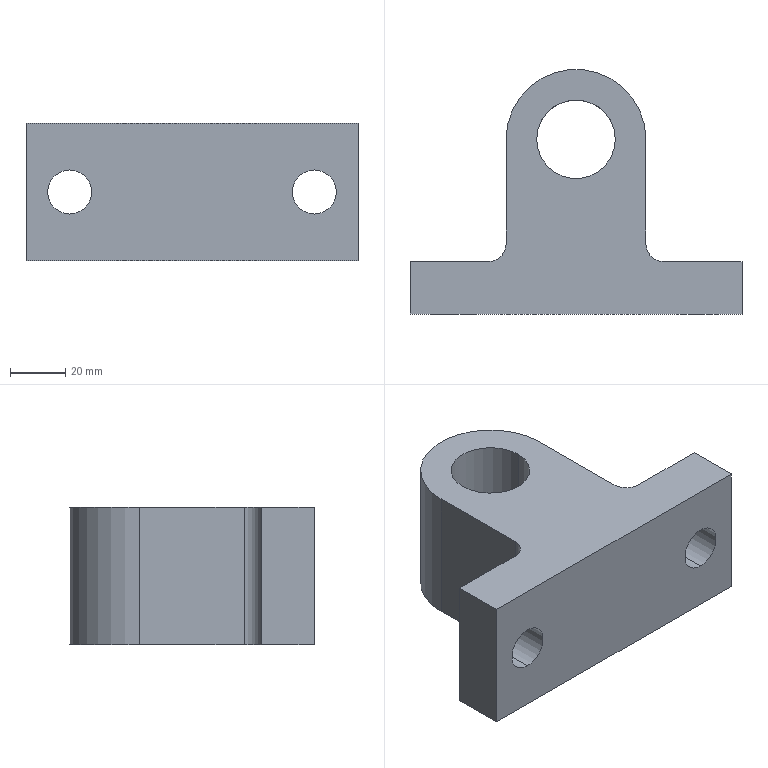Part | SolidWorks | features Cut 1, Extrusion 1, Fillet 1 | 1 solid | 18 faces | box 120.65 x 88.9 x 50 mm | volume 239631 mm3 | cylinder 9 | plane 9 | commonest cylinder face diameters 16.002 x4 12.7 x2 28.575 x2 50.8 x1
STEP:
#1=CARTESIAN_POINT('',(-44.45,-63.5,-8.001));
#2=VERTEX_POINT('',#1);
#3=CARTESIAN_POINT('',(-44.45,-63.5,8.001));
#4=VERTEX_POINT('',#3);
#5=CARTESIAN_POINT('',(-44.45,-63.5,0.));
#6=DIRECTION('',(0.,1.,0.));
#7=DIRECTION('',(0.,0.,-1.));
#8=AXIS2_PLACEMENT_3D('',#5,#6,#7);
#9=CIRCLE('',#8,8.001);
#10=EDGE_CURVE('',#2,#4,#9,.T.);
#11=ORIENTED_EDGE('',*,*,#10,.F.);
#12=CARTESIAN_POINT('',(-44.45,-44.45,-8.001));
#13=VERTEX_POINT('',#12);
#14=CARTESIAN_POINT('',(-44.45,-63.5,-8.001));
#15=DIRECTION('',(0.,1.,0.));
#16=VECTOR('',#15,1000.);
#17=LINE('',#14,#16);
#18=EDGE_CURVE('',#2,#13,#17,.T.);
#19=ORIENTED_EDGE('',*,*,#18,.T.);
#20=CARTESIAN_POINT('',(-44.45,-44.45,8.001));
#21=VERTEX_POINT('',#20);
#22=CARTESIAN_POINT('',(-44.45,-44.45,0.));
#23=DIRECTION('',(0.,-1.,0.));
#24=DIRECTION('',(0.,0.,-1.));
#25=AXIS2_PLACEMENT_3D('',#22,#23,#24);
#26=CIRCLE('',#25,8.001);
#27=EDGE_CURVE('',#21,#13,#26,.T.);
#28=ORIENTED_EDGE('',*,*,#27,.F.);
#29=CARTESIAN_POINT('',(-44.45,-63.5,8.001));
#30=DIRECTION('',(0.,1.,0.));
#31=VECTOR('',#30,1000.);
#32=LINE('',#29,#31);
#33=EDGE_CURVE('',#4,#21,#32,.T.);
#34=ORIENTED_EDGE('',*,*,#33,.F.);
#35=EDGE_LOOP('',(#11,#19,#28,#34));
#36=FACE_OUTER_BOUND('',#35,.T.);
#37=CARTESIAN_POINT('',(-44.45,-63.5,0.));
#38=DIRECTION('',(0.,1.,0.));
#39=DIRECTION('',(0.,0.,1.));
#40=AXIS2_PLACEMENT_3D('',#37,#38,#39);
#41=CYLINDRICAL_SURFACE('',#40,8.001);
#42=ADVANCED_FACE('',(#36),#41,.F.);
#43=CARTESIAN_POINT('',(44.45,-63.5,-8.001));
#44=VERTEX_POINT('',#43);
#45=CARTESIAN_POINT('',(44.45,-63.5,8.001));
#46=VERTEX_POINT('',#45);
#47=CARTESIAN_POINT('',(44.45,-63.5,0.));
#48=DIRECTION('',(0.,1.,0.));
#49=DIRECTION('',(0.,0.,1.));
#50=AXIS2_PLACEMENT_3D('',#47,#48,#49);
#51=CIRCLE('',#50,8.001);
#52=EDGE_CURVE('',#44,#46,#51,.T.);
#53=ORIENTED_EDGE('',*,*,#52,.F.);
#54=CARTESIAN_POINT('',(44.45,-44.45,-8.001));
#55=VERTEX_POINT('',#54);
#56=CARTESIAN_POINT('',(44.45,-63.5,-8.001));
#57=DIRECTION('',(0.,1.,0.));
#58=VECTOR('',#57,1000.);
#59=LINE('',#56,#58);
#60=EDGE_CURVE('',#44,#55,#59,.T.);
#61=ORIENTED_EDGE('',*,*,#60,.T.);
#62=CARTESIAN_POINT('',(44.45,-44.45,8.001));
#63=VERTEX_POINT('',#62);
#64=CARTESIAN_POINT('',(44.45,-44.45,0.));
#65=DIRECTION('',(0.,-1.,0.));
#66=DIRECTION('',(1.,0.,0.));
#67=AXIS2_PLACEMENT_3D('',#64,#65,#66);
#68=CIRCLE('',#67,8.001);
#69=EDGE_CURVE('',#63,#55,#68,.T.);
#70=ORIENTED_EDGE('',*,*,#69,.F.);
#71=CARTESIAN_POINT('',(44.45,-63.5,8.001));
#72=DIRECTION('',(0.,1.,0.));
#73=VECTOR('',#72,1000.);
#74=LINE('',#71,#73);
#75=EDGE_CURVE('',#46,#63,#74,.T.);
#76=ORIENTED_EDGE('',*,*,#75,.F.);
#77=EDGE_LOOP('',(#53,#61,#70,#76));
#78=FACE_OUTER_BOUND('',#77,.T.);
#79=CARTESIAN_POINT('',(44.45,-63.5,0.));
#80=DIRECTION('',(0.,1.,0.));
#81=DIRECTION('',(0.,0.,1.));
#82=AXIS2_PLACEMENT_3D('',#79,#80,#81);
#83=CYLINDRICAL_SURFACE('',#82,8.001);
#84=ADVANCED_FACE('',(#78),#83,.F.);
#85=CARTESIAN_POINT('',(-14.288,0.,25.));
#86=VERTEX_POINT('',#85);
#87=CARTESIAN_POINT('',(14.288,0.,25.));
#88=VERTEX_POINT('',#87);
#89=CARTESIAN_POINT('',(0.,0.,25.));
#90=DIRECTION('',(0.,0.,1.));
#91=DIRECTION('',(1.,0.,0.));
#92=AXIS2_PLACEMENT_3D('',#89,#90,#91);
#93=CIRCLE('',#92,14.288);
#94=EDGE_CURVE('',#86,#88,#93,.T.);
#95=ORIENTED_EDGE('',*,*,#94,.T.);
#96=CARTESIAN_POINT('',(14.288,0.,-25.));
#97=VERTEX_POINT('',#96);
#98=CARTESIAN_POINT('',(14.288,0.,25.));
#99=DIRECTION('',(0.,0.,-1.));
#100=VECTOR('',#99,1000.);
#101=LINE('',#98,#100);
#102=EDGE_CURVE('',#88,#97,#101,.T.);
#103=ORIENTED_EDGE('',*,*,#102,.T.);
#104=CARTESIAN_POINT('',(-14.288,0.,-25.));
#105=VERTEX_POINT('',#104);
#106=CARTESIAN_POINT('',(0.,0.,-25.));
#107=DIRECTION('',(0.,0.,1.));
#108=DIRECTION('',(1.,0.,0.));
#109=AXIS2_PLACEMENT_3D('',#106,#107,#108);
#110=CIRCLE('',#109,14.288);
#111=EDGE_CURVE('',#105,#97,#110,.T.);
#112=ORIENTED_EDGE('',*,*,#111,.F.);
#113=CARTESIAN_POINT('',(-14.288,0.,25.));
#114=DIRECTION('',(0.,0.,-1.));
#115=VECTOR('',#114,1000.);
#116=LINE('',#113,#115);
#117=EDGE_CURVE('',#86,#105,#116,.T.);
#118=ORIENTED_EDGE('',*,*,#117,.F.);
#119=EDGE_LOOP('',(#95,#103,#112,#118));
#120=FACE_OUTER_BOUND('',#119,.T.);
#121=CARTESIAN_POINT('',(0.,0.,25.));
#122=DIRECTION('',(0.,0.,-1.));
#123=DIRECTION('',(-1.,0.,0.));
#124=AXIS2_PLACEMENT_3D('',#121,#122,#123);
#125=CYLINDRICAL_SURFACE('',#124,14.288);
#126=ADVANCED_FACE('',(#120),#125,.F.);
#127=CARTESIAN_POINT('',(25.4,0.,25.));
#128=VERTEX_POINT('',#127);
#129=CARTESIAN_POINT('',(-25.4,0.,25.));
#130=VERTEX_POINT('',#129);
#131=CARTESIAN_POINT('',(0.,0.,25.));
#132=DIRECTION('',(0.,0.,1.));
#133=DIRECTION('',(1.,0.,0.));
#134=AXIS2_PLACEMENT_3D('',#131,#132,#133);
#135=CIRCLE('',#134,25.4);
#136=EDGE_CURVE('',#128,#130,#135,.T.);
#137=ORIENTED_EDGE('',*,*,#136,.T.);
#138=CARTESIAN_POINT('',(-25.4,-38.1,25.));
#139=VERTEX_POINT('',#138);
#140=CARTESIAN_POINT('',(-25.4,0.,25.));
#141=DIRECTION('',(0.,-1.,0.));
#142=VECTOR('',#141,1000.);
#143=LINE('',#140,#142);
#144=EDGE_CURVE('',#130,#139,#143,.T.);
#145=ORIENTED_EDGE('',*,*,#144,.T.);
#146=CARTESIAN_POINT('',(-31.75,-44.45,25.));
#147=VERTEX_POINT('',#146);
#148=CARTESIAN_POINT('',(-31.75,-38.1,25.));
#149=DIRECTION('',(0.,0.,-1.));
#150=DIRECTION('',(1.,0.,0.));
#151=AXIS2_PLACEMENT_3D('',#148,#149,#150);
#152=CIRCLE('',#151,6.35);
#153=EDGE_CURVE('',#139,#147,#152,.T.);
#154=ORIENTED_EDGE('',*,*,#153,.T.);
#155=CARTESIAN_POINT('',(-60.325,-44.45,25.));
#156=VERTEX_POINT('',#155);
#157=CARTESIAN_POINT('',(-25.4,-44.45,25.));
#158=DIRECTION('',(-1.,0.,0.));
#159=VECTOR('',#158,1000.);
#160=LINE('',#157,#159);
#161=EDGE_CURVE('',#147,#156,#160,.T.);
#162=ORIENTED_EDGE('',*,*,#161,.T.);
#163=CARTESIAN_POINT('',(-60.325,-63.5,25.));
#164=VERTEX_POINT('',#163);
#165=CARTESIAN_POINT('',(-60.325,-44.45,25.));
#166=DIRECTION('',(0.,-1.,0.));
#167=VECTOR('',#166,1000.);
#168=LINE('',#165,#167);
#169=EDGE_CURVE('',#156,#164,#168,.T.);
#170=ORIENTED_EDGE('',*,*,#169,.T.);
#171=CARTESIAN_POINT('',(60.325,-63.5,25.));
#172=VERTEX_POINT('',#171);
#173=CARTESIAN_POINT('',(-60.325,-63.5,25.));
#174=DIRECTION('',(1.,0.,0.));
#175=VECTOR('',#174,1000.);
#176=LINE('',#173,#175);
#177=EDGE_CURVE('',#164,#172,#176,.T.);
#178=ORIENTED_EDGE('',*,*,#177,.T.);
#179=CARTESIAN_POINT('',(60.325,-44.45,25.));
#180=VERTEX_POINT('',#179);
#181=CARTESIAN_POINT('',(60.325,-44.45,25.));
#182=DIRECTION('',(0.,1.,0.));
#183=VECTOR('',#182,1000.);
#184=LINE('',#181,#183);
#185=EDGE_CURVE('',#172,#180,#184,.T.);
#186=ORIENTED_EDGE('',*,*,#185,.T.);
#187=CARTESIAN_POINT('',(31.75,-44.45,25.));
#188=VERTEX_POINT('',#187);
#189=CARTESIAN_POINT('',(25.4,-44.45,25.));
#190=DIRECTION('',(-1.,0.,0.));
#191=VECTOR('',#190,1000.);
#192=LINE('',#189,#191);
#193=EDGE_CURVE('',#180,#188,#192,.T.);
#194=ORIENTED_EDGE('',*,*,#193,.T.);
#195=CARTESIAN_POINT('',(25.4,-38.1,25.));
#196=VERTEX_POINT('',#195);
#197=CARTESIAN_POINT('',(31.75,-38.1,25.));
#198=DIRECTION('',(0.,0.,-1.));
#199=DIRECTION('',(1.,0.,0.));
#200=AXIS2_PLACEMENT_3D('',#197,#198,#199);
#201=CIRCLE('',#200,6.35);
#202=EDGE_CURVE('',#188,#196,#201,.T.);
#203=ORIENTED_EDGE('',*,*,#202,.T.);
#204=CARTESIAN_POINT('',(25.4,0.,25.));
#205=DIRECTION('',(0.,1.,0.));
#206=VECTOR('',#205,1000.);
#207=LINE('',#204,#206);
#208=EDGE_CURVE('',#196,#128,#207,.T.);
#209=ORIENTED_EDGE('',*,*,#208,.T.);
#210=EDGE_LOOP('',(#137,#145,#154,#162,#170,#178,#186,#194,#203,#209));
#211=FACE_OUTER_BOUND('',#210,.T.);
#212=ORIENTED_EDGE('',*,*,#94,.F.);
#213=CARTESIAN_POINT('',(0.,0.,25.));
#214=DIRECTION('',(0.,0.,1.));
#215=DIRECTION('',(1.,0.,0.));
#216=AXIS2_PLACEMENT_3D('',#213,#214,#215);
#217=CIRCLE('',#216,14.288);
#218=EDGE_CURVE('',#88,#86,#217,.T.);
#219=ORIENTED_EDGE('',*,*,#218,.F.);
#220=EDGE_LOOP('',(#212,#219));
#221=FACE_BOUND('',#220,.T.);
#222=CARTESIAN_POINT('',(0.,0.,25.));
#223=DIRECTION('',(0.,0.,1.));
#224=DIRECTION('',(1.,0.,0.));
#225=AXIS2_PLACEMENT_3D('',#222,#223,#224);
#226=PLANE('',#225);
#227=ADVANCED_FACE('',(#211,#221),#226,.T.);
#228=CARTESIAN_POINT('',(25.4,0.,-25.));
#229=VERTEX_POINT('',#228);
#230=CARTESIAN_POINT('',(-25.4,0.,-25.));
#231=VERTEX_POINT('',#230);
#232=CARTESIAN_POINT('',(0.,0.,-25.));
#233=DIRECTION('',(0.,0.,1.));
#234=DIRECTION('',(1.,0.,0.));
#235=AXIS2_PLACEMENT_3D('',#232,#233,#234);
#236=CIRCLE('',#235,25.4);
#237=EDGE_CURVE('',#229,#231,#236,.T.);
#238=ORIENTED_EDGE('',*,*,#237,.F.);
#239=CARTESIAN_POINT('',(25.4,-38.1,-25.));
#240=VERTEX_POINT('',#239);
#241=CARTESIAN_POINT('',(25.4,0.,-25.));
#242=DIRECTION('',(0.,1.,0.));
#243=VECTOR('',#242,1000.);
#244=LINE('',#241,#243);
#245=EDGE_CURVE('',#240,#229,#244,.T.);
#246=ORIENTED_EDGE('',*,*,#245,.F.);
#247=CARTESIAN_POINT('',(31.75,-44.45,-25.));
#248=VERTEX_POINT('',#247);
#249=CARTESIAN_POINT('',(31.75,-38.1,-25.));
#250=DIRECTION('',(0.,0.,1.));
#251=DIRECTION('',(1.,0.,0.));
#252=AXIS2_PLACEMENT_3D('',#249,#250,#251);
#253=CIRCLE('',#252,6.35);
#254=EDGE_CURVE('',#240,#248,#253,.T.);
#255=ORIENTED_EDGE('',*,*,#254,.T.);
#256=CARTESIAN_POINT('',(60.325,-44.45,-25.));
#257=VERTEX_POINT('',#256);
#258=CARTESIAN_POINT('',(25.4,-44.45,-25.));
#259=DIRECTION('',(-1.,0.,0.));
#260=VECTOR('',#259,1000.);
#261=LINE('',#258,#260);
#262=EDGE_CURVE('',#257,#248,#261,.T.);
#263=ORIENTED_EDGE('',*,*,#262,.F.);
#264=CARTESIAN_POINT('',(60.325,-63.5,-25.));
#265=VERTEX_POINT('',#264);
#266=CARTESIAN_POINT('',(60.325,-44.45,-25.));
#267=DIRECTION('',(0.,1.,0.));
#268=VECTOR('',#267,1000.);
#269=LINE('',#266,#268);
#270=EDGE_CURVE('',#265,#257,#269,.T.);
#271=ORIENTED_EDGE('',*,*,#270,.F.);
#272=CARTESIAN_POINT('',(-60.325,-63.5,-25.));
#273=VERTEX_POINT('',#272);
#274=CARTESIAN_POINT('',(-60.325,-63.5,-25.));
#275=DIRECTION('',(1.,0.,0.));
#276=VECTOR('',#275,1000.);
#277=LINE('',#274,#276);
#278=EDGE_CURVE('',#273,#265,#277,.T.);
#279=ORIENTED_EDGE('',*,*,#278,.F.);
#280=CARTESIAN_POINT('',(-60.325,-44.45,-25.));
#281=VERTEX_POINT('',#280);
#282=CARTESIAN_POINT('',(-60.325,-44.45,-25.));
#283=DIRECTION('',(0.,-1.,0.));
#284=VECTOR('',#283,1000.);
#285=LINE('',#282,#284);
#286=EDGE_CURVE('',#281,#273,#285,.T.);
#287=ORIENTED_EDGE('',*,*,#286,.F.);
#288=CARTESIAN_POINT('',(-31.75,-44.45,-25.));
#289=VERTEX_POINT('',#288);
#290=CARTESIAN_POINT('',(-25.4,-44.45,-25.));
#291=DIRECTION('',(-1.,0.,0.));
#292=VECTOR('',#291,1000.);
#293=LINE('',#290,#292);
#294=EDGE_CURVE('',#289,#281,#293,.T.);
#295=ORIENTED_EDGE('',*,*,#294,.F.);
#296=CARTESIAN_POINT('',(-25.4,-38.1,-25.));
#297=VERTEX_POINT('',#296);
#298=CARTESIAN_POINT('',(-31.75,-38.1,-25.));
#299=DIRECTION('',(0.,0.,1.));
#300=DIRECTION('',(1.,0.,0.));
#301=AXIS2_PLACEMENT_3D('',#298,#299,#300);
#302=CIRCLE('',#301,6.35);
#303=EDGE_CURVE('',#289,#297,#302,.T.);
#304=ORIENTED_EDGE('',*,*,#303,.T.);
#305=CARTESIAN_POINT('',(-25.4,0.,-25.));
#306=DIRECTION('',(0.,-1.,0.));
#307=VECTOR('',#306,1000.);
#308=LINE('',#305,#307);
#309=EDGE_CURVE('',#231,#297,#308,.T.);
#310=ORIENTED_EDGE('',*,*,#309,.F.);
#311=EDGE_LOOP('',(#238,#246,#255,#263,#271,#279,#287,#295,#304,#310));
#312=FACE_OUTER_BOUND('',#311,.T.);
#313=ORIENTED_EDGE('',*,*,#111,.T.);
#314=CARTESIAN_POINT('',(0.,0.,-25.));
#315=DIRECTION('',(0.,0.,1.));
#316=DIRECTION('',(1.,0.,0.));
#317=AXIS2_PLACEMENT_3D('',#314,#315,#316);
#318=CIRCLE('',#317,14.288);
#319=EDGE_CURVE('',#97,#105,#318,.T.);
#320=ORIENTED_EDGE('',*,*,#319,.T.);
#321=EDGE_LOOP('',(#313,#320));
#322=FACE_BOUND('',#321,.T.);
#323=CARTESIAN_POINT('',(0.,0.,-25.));
#324=DIRECTION('',(0.,0.,1.));
#325=DIRECTION('',(1.,0.,0.));
#326=AXIS2_PLACEMENT_3D('',#323,#324,#325);
#327=PLANE('',#326);
#328=ADVANCED_FACE('',(#312,#322),#327,.F.);
#329=ORIENTED_EDGE('',*,*,#237,.T.);
#330=CARTESIAN_POINT('',(-25.4,0.,25.));
#331=DIRECTION('',(0.,0.,-1.));
#332=VECTOR('',#331,1000.);
#333=LINE('',#330,#332);
#334=EDGE_CURVE('',#130,#231,#333,.T.);
#335=ORIENTED_EDGE('',*,*,#334,.F.);
#336=ORIENTED_EDGE('',*,*,#136,.F.);
#337=CARTESIAN_POINT('',(25.4,0.,25.));
#338=DIRECTION('',(0.,0.,-1.));
#339=VECTOR('',#338,1000.);
#340=LINE('',#337,#339);
#341=EDGE_CURVE('',#128,#229,#340,.T.);
#342=ORIENTED_EDGE('',*,*,#341,.T.);
#343=EDGE_LOOP('',(#329,#335,#336,#342));
#344=FACE_OUTER_BOUND('',#343,.T.);
#345=CARTESIAN_POINT('',(0.,0.,25.));
#346=DIRECTION('',(0.,0.,-1.));
#347=DIRECTION('',(-1.,0.,0.));
#348=AXIS2_PLACEMENT_3D('',#345,#346,#347);
#349=CYLINDRICAL_SURFACE('',#348,25.4);
#350=ADVANCED_FACE('',(#344),#349,.T.);
#351=ORIENTED_EDGE('',*,*,#309,.T.);
#352=CARTESIAN_POINT('',(-25.4,-38.1,25.));
#353=DIRECTION('',(0.,0.,1.));
#354=VECTOR('',#353,1000.);
#355=LINE('',#352,#354);
#356=EDGE_CURVE('',#297,#139,#355,.T.);
#357=ORIENTED_EDGE('',*,*,#356,.T.);
#358=ORIENTED_EDGE('',*,*,#144,.F.);
#359=ORIENTED_EDGE('',*,*,#334,.T.);
#360=EDGE_LOOP('',(#351,#357,#358,#359));
#361=FACE_OUTER_BOUND('',#360,.T.);
#362=CARTESIAN_POINT('',(-25.4,0.,25.));
#363=DIRECTION('',(1.,0.,0.));
#364=DIRECTION('',(0.,1.,0.));
#365=AXIS2_PLACEMENT_3D('',#362,#363,#364);
#366=PLANE('',#365);
#367=ADVANCED_FACE('',(#361),#366,.F.);
#368=ORIENTED_EDGE('',*,*,#27,.T.);
#369=CARTESIAN_POINT('',(-44.45,-44.45,0.));
#370=DIRECTION('',(0.,-1.,0.));
#371=DIRECTION('',(0.,0.,-1.));
#372=AXIS2_PLACEMENT_3D('',#369,#370,#371);
#373=CIRCLE('',#372,8.001);
#374=EDGE_CURVE('',#13,#21,#373,.T.);
#375=ORIENTED_EDGE('',*,*,#374,.T.);
#376=EDGE_LOOP('',(#368,#375));
#377=FACE_BOUND('',#376,.T.);
#378=ORIENTED_EDGE('',*,*,#161,.F.);
#379=CARTESIAN_POINT('',(-31.75,-44.45,-25.));
#380=DIRECTION('',(0.,0.,-1.));
#381=VECTOR('',#380,1000.);
#382=LINE('',#379,#381);
#383=EDGE_CURVE('',#147,#289,#382,.T.);
#384=ORIENTED_EDGE('',*,*,#383,.T.);
#385=ORIENTED_EDGE('',*,*,#294,.T.);
#386=CARTESIAN_POINT('',(-60.325,-44.45,25.));
#387=DIRECTION('',(0.,0.,-1.));
#388=VECTOR('',#387,1000.);
#389=LINE('',#386,#388);
#390=EDGE_CURVE('',#156,#281,#389,.T.);
#391=ORIENTED_EDGE('',*,*,#390,.F.);
#392=EDGE_LOOP('',(#378,#384,#385,#391));
#393=FACE_OUTER_BOUND('',#392,.T.);
#394=CARTESIAN_POINT('',(-25.4,-44.45,25.));
#395=DIRECTION('',(0.,-1.,0.));
#396=DIRECTION('',(0.,0.,-1.));
#397=AXIS2_PLACEMENT_3D('',#394,#395,#396);
#398=PLANE('',#397);
#399=ADVANCED_FACE('',(#377,#393),#398,.F.);
#400=ORIENTED_EDGE('',*,*,#286,.T.);
#401=CARTESIAN_POINT('',(-60.325,-63.5,25.));
#402=DIRECTION('',(0.,0.,-1.));
#403=VECTOR('',#402,1000.);
#404=LINE('',#401,#403);
#405=EDGE_CURVE('',#164,#273,#404,.T.);
#406=ORIENTED_EDGE('',*,*,#405,.F.);
#407=ORIENTED_EDGE('',*,*,#169,.F.);
#408=ORIENTED_EDGE('',*,*,#390,.T.);
#409=EDGE_LOOP('',(#400,#406,#407,#408));
#410=FACE_OUTER_BOUND('',#409,.T.);
#411=CARTESIAN_POINT('',(-60.325,-44.45,25.));
#412=DIRECTION('',(1.,0.,0.));
#413=DIRECTION('',(0.,0.,-1.));
#414=AXIS2_PLACEMENT_3D('',#411,#412,#413);
#415=PLANE('',#414);
#416=ADVANCED_FACE('',(#410),#415,.F.);
#417=CARTESIAN_POINT('',(-44.45,-63.5,0.));
#418=DIRECTION('',(0.,1.,0.));
#419=DIRECTION('',(0.,0.,-1.));
#420=AXIS2_PLACEMENT_3D('',#417,#418,#419);
#421=CIRCLE('',#420,8.001);
#422=EDGE_CURVE('',#4,#2,#421,.T.);
#423=ORIENTED_EDGE('',*,*,#422,.T.);
#424=ORIENTED_EDGE('',*,*,#10,.T.);
#425=EDGE_LOOP('',(#423,#424));
#426=FACE_BOUND('',#425,.T.);
#427=CARTESIAN_POINT('',(44.45,-63.5,0.));
#428=DIRECTION('',(0.,1.,0.));
#429=DIRECTION('',(0.,0.,1.));
#430=AXIS2_PLACEMENT_3D('',#427,#428,#429);
#431=CIRCLE('',#430,8.001);
#432=EDGE_CURVE('',#46,#44,#431,.T.);
#433=ORIENTED_EDGE('',*,*,#432,.T.);
#434=ORIENTED_EDGE('',*,*,#52,.T.);
#435=EDGE_LOOP('',(#433,#434));
#436=FACE_BOUND('',#435,.T.);
#437=ORIENTED_EDGE('',*,*,#278,.T.);
#438=CARTESIAN_POINT('',(60.325,-63.5,25.));
#439=DIRECTION('',(0.,0.,-1.));
#440=VECTOR('',#439,1000.);
#441=LINE('',#438,#440);
#442=EDGE_CURVE('',#172,#265,#441,.T.);
#443=ORIENTED_EDGE('',*,*,#442,.F.);
#444=ORIENTED_EDGE('',*,*,#177,.F.);
#445=ORIENTED_EDGE('',*,*,#405,.T.);
#446=EDGE_LOOP('',(#437,#443,#444,#445));
#447=FACE_OUTER_BOUND('',#446,.T.);
#448=CARTESIAN_POINT('',(-60.325,-63.5,25.));
#449=DIRECTION('',(0.,1.,0.));
#450=DIRECTION('',(-1.,0.,0.));
#451=AXIS2_PLACEMENT_3D('',#448,#449,#450);
#452=PLANE('',#451);
#453=ADVANCED_FACE('',(#426,#436,#447),#452,.F.);
#454=ORIENTED_EDGE('',*,*,#270,.T.);
#455=CARTESIAN_POINT('',(60.325,-44.45,25.));
#456=DIRECTION('',(0.,0.,-1.));
#457=VECTOR('',#456,1000.);
#458=LINE('',#455,#457);
#459=EDGE_CURVE('',#180,#257,#458,.T.);
#460=ORIENTED_EDGE('',*,*,#459,.F.);
#461=ORIENTED_EDGE('',*,*,#185,.F.);
#462=ORIENTED_EDGE('',*,*,#442,.T.);
#463=EDGE_LOOP('',(#454,#460,#461,#462));
#464=FACE_OUTER_BOUND('',#463,.T.);
#465=CARTESIAN_POINT('',(60.325,-44.45,25.));
#466=DIRECTION('',(-1.,0.,0.));
#467=DIRECTION('',(0.,0.,1.));
#468=AXIS2_PLACEMENT_3D('',#465,#466,#467);
#469=PLANE('',#468);
#470=ADVANCED_FACE('',(#464),#469,.F.);
#471=ORIENTED_EDGE('',*,*,#69,.T.);
#472=CARTESIAN_POINT('',(44.45,-44.45,0.));
#473=DIRECTION('',(0.,-1.,0.));
#474=DIRECTION('',(1.,0.,0.));
#475=AXIS2_PLACEMENT_3D('',#472,#473,#474);
#476=CIRCLE('',#475,8.001);
#477=EDGE_CURVE('',#55,#63,#476,.T.);
#478=ORIENTED_EDGE('',*,*,#477,.T.);
#479=EDGE_LOOP('',(#471,#478));
#480=FACE_BOUND('',#479,.T.);
#481=ORIENTED_EDGE('',*,*,#262,.T.);
#482=CARTESIAN_POINT('',(31.75,-44.45,25.));
#483=DIRECTION('',(0.,0.,1.));
#484=VECTOR('',#483,1000.);
#485=LINE('',#482,#484);
#486=EDGE_CURVE('',#248,#188,#485,.T.);
#487=ORIENTED_EDGE('',*,*,#486,.T.);
#488=ORIENTED_EDGE('',*,*,#193,.F.);
#489=ORIENTED_EDGE('',*,*,#459,.T.);
#490=EDGE_LOOP('',(#481,#487,#488,#489));
#491=FACE_OUTER_BOUND('',#490,.T.);
#492=CARTESIAN_POINT('',(25.4,-44.45,25.));
#493=DIRECTION('',(0.,-1.,0.));
#494=DIRECTION('',(1.,0.,0.));
#495=AXIS2_PLACEMENT_3D('',#492,#493,#494);
#496=PLANE('',#495);
#497=ADVANCED_FACE('',(#480,#491),#496,.F.);
#498=ORIENTED_EDGE('',*,*,#208,.F.);
#499=CARTESIAN_POINT('',(25.4,-38.1,-25.));
#500=DIRECTION('',(0.,0.,-1.));
#501=VECTOR('',#500,1000.);
#502=LINE('',#499,#501);
#503=EDGE_CURVE('',#196,#240,#502,.T.);
#504=ORIENTED_EDGE('',*,*,#503,.T.);
#505=ORIENTED_EDGE('',*,*,#245,.T.);
#506=ORIENTED_EDGE('',*,*,#341,.F.);
#507=EDGE_LOOP('',(#498,#504,#505,#506));
#508=FACE_OUTER_BOUND('',#507,.T.);
#509=CARTESIAN_POINT('',(25.4,0.,25.));
#510=DIRECTION('',(-1.,0.,0.));
#511=DIRECTION('',(0.,-1.,0.));
#512=AXIS2_PLACEMENT_3D('',#509,#510,#511);
#513=PLANE('',#512);
#514=ADVANCED_FACE('',(#508),#513,.F.);
#515=ORIENTED_EDGE('',*,*,#102,.F.);
#516=ORIENTED_EDGE('',*,*,#218,.T.);
#517=ORIENTED_EDGE('',*,*,#117,.T.);
#518=ORIENTED_EDGE('',*,*,#319,.F.);
#519=EDGE_LOOP('',(#515,#516,#517,#518));
#520=FACE_OUTER_BOUND('',#519,.T.);
#521=CARTESIAN_POINT('',(0.,0.,25.));
#522=DIRECTION('',(0.,0.,-1.));
#523=DIRECTION('',(-1.,0.,0.));
#524=AXIS2_PLACEMENT_3D('',#521,#522,#523);
#525=CYLINDRICAL_SURFACE('',#524,14.288);
#526=ADVANCED_FACE('',(#520),#525,.F.);
#527=ORIENTED_EDGE('',*,*,#202,.F.);
#528=ORIENTED_EDGE('',*,*,#486,.F.);
#529=ORIENTED_EDGE('',*,*,#254,.F.);
#530=ORIENTED_EDGE('',*,*,#503,.F.);
#531=EDGE_LOOP('',(#527,#528,#529,#530));
#532=FACE_OUTER_BOUND('',#531,.T.);
#533=CARTESIAN_POINT('',(31.75,-38.1,25.));
#534=DIRECTION('',(0.,0.,1.));
#535=DIRECTION('',(1.,0.,0.));
#536=AXIS2_PLACEMENT_3D('',#533,#534,#535);
#537=CYLINDRICAL_SURFACE('',#536,6.35);
#538=ADVANCED_FACE('',(#532),#537,.F.);
#539=ORIENTED_EDGE('',*,*,#153,.F.);
#540=ORIENTED_EDGE('',*,*,#356,.F.);
#541=ORIENTED_EDGE('',*,*,#303,.F.);
#542=ORIENTED_EDGE('',*,*,#383,.F.);
#543=EDGE_LOOP('',(#539,#540,#541,#542));
#544=FACE_OUTER_BOUND('',#543,.T.);
#545=CARTESIAN_POINT('',(-31.75,-38.1,25.));
#546=DIRECTION('',(0.,0.,1.));
#547=DIRECTION('',(1.,0.,0.));
#548=AXIS2_PLACEMENT_3D('',#545,#546,#547);
#549=CYLINDRICAL_SURFACE('',#548,6.35);
#550=ADVANCED_FACE('',(#544),#549,.F.);
#551=ORIENTED_EDGE('',*,*,#60,.F.);
#552=ORIENTED_EDGE('',*,*,#432,.F.);
#553=ORIENTED_EDGE('',*,*,#75,.T.);
#554=ORIENTED_EDGE('',*,*,#477,.F.);
#555=EDGE_LOOP('',(#551,#552,#553,#554));
#556=FACE_OUTER_BOUND('',#555,.T.);
#557=CARTESIAN_POINT('',(44.45,-63.5,0.));
#558=DIRECTION('',(0.,1.,0.));
#559=DIRECTION('',(0.,0.,1.));
#560=AXIS2_PLACEMENT_3D('',#557,#558,#559);
#561=CYLINDRICAL_SURFACE('',#560,8.001);
#562=ADVANCED_FACE('',(#556),#561,.F.);
#563=ORIENTED_EDGE('',*,*,#18,.F.);
#564=ORIENTED_EDGE('',*,*,#422,.F.);
#565=ORIENTED_EDGE('',*,*,#33,.T.);
#566=ORIENTED_EDGE('',*,*,#374,.F.);
#567=EDGE_LOOP('',(#563,#564,#565,#566));
#568=FACE_OUTER_BOUND('',#567,.T.);
#569=CARTESIAN_POINT('',(-44.45,-63.5,0.));
#570=DIRECTION('',(0.,1.,0.));
#571=DIRECTION('',(0.,0.,1.));
#572=AXIS2_PLACEMENT_3D('',#569,#570,#571);
#573=CYLINDRICAL_SURFACE('',#572,8.001);
#574=ADVANCED_FACE('',(#568),#573,.F.);
#575=CLOSED_SHELL('',(#42,#84,#126,#227,#328,#350,#367,#399,#416,#453,#470,#497,#514,#526,#538,#550,#562,#574));
#576=MANIFOLD_SOLID_BREP('',#575);
#577=CARTESIAN_POINT('',(0.,0.,0.));
#578=DIRECTION('',(0.,0.,1.));
#579=DIRECTION('',(1.,0.,0.));
#580=AXIS2_PLACEMENT_3D('',#577,#578,#579);
#581=(LENGTH_UNIT()NAMED_UNIT(*)SI_UNIT(.MILLI.,.METRE.));
#582=UNCERTAINTY_MEASURE_WITH_UNIT(LENGTH_MEASURE(0.00001),#581,'','');
#583=(NAMED_UNIT(*)PLANE_ANGLE_UNIT()SI_UNIT($,.RADIAN.));
#584=(NAMED_UNIT(*)SI_UNIT($,.STERADIAN.)SOLID_ANGLE_UNIT());
#585=(GEOMETRIC_REPRESENTATION_CONTEXT(3)GLOBAL_UNCERTAINTY_ASSIGNED_CONTEXT((#582))GLOBAL_UNIT_ASSIGNED_CONTEXT((#581,#583,#584))REPRESENTATION_CONTEXT('',''));
#586=ADVANCED_BREP_SHAPE_REPRESENTATION('',(#576,#580),#585);